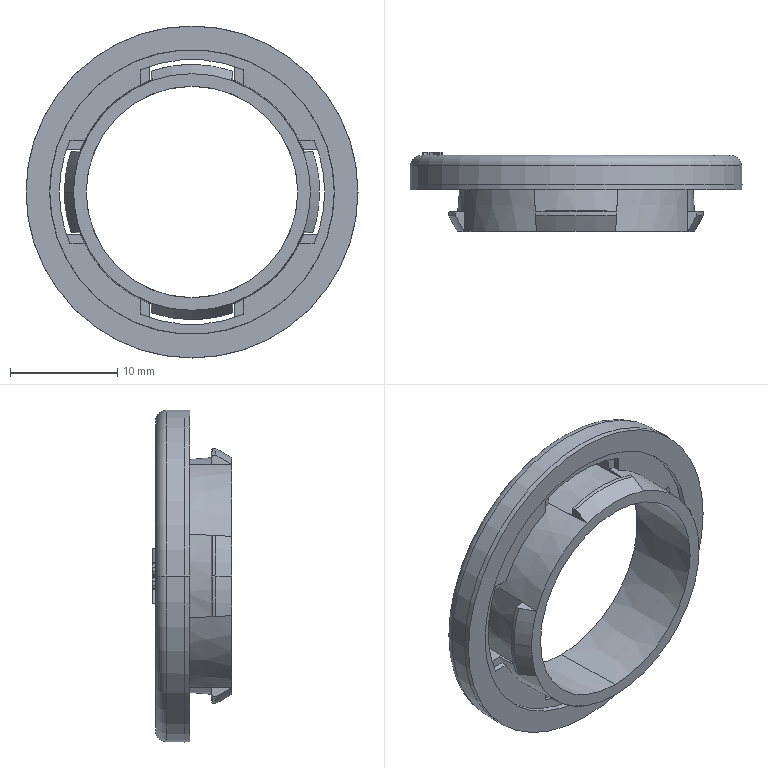Part | STEP file | MSBR-26 | 1 solid | 124 faces | box 31 x 7.4 x 31 mm | volume 1482 mm3 | plane 74 | cone 32 | other 12 | spline 4 | torus 2